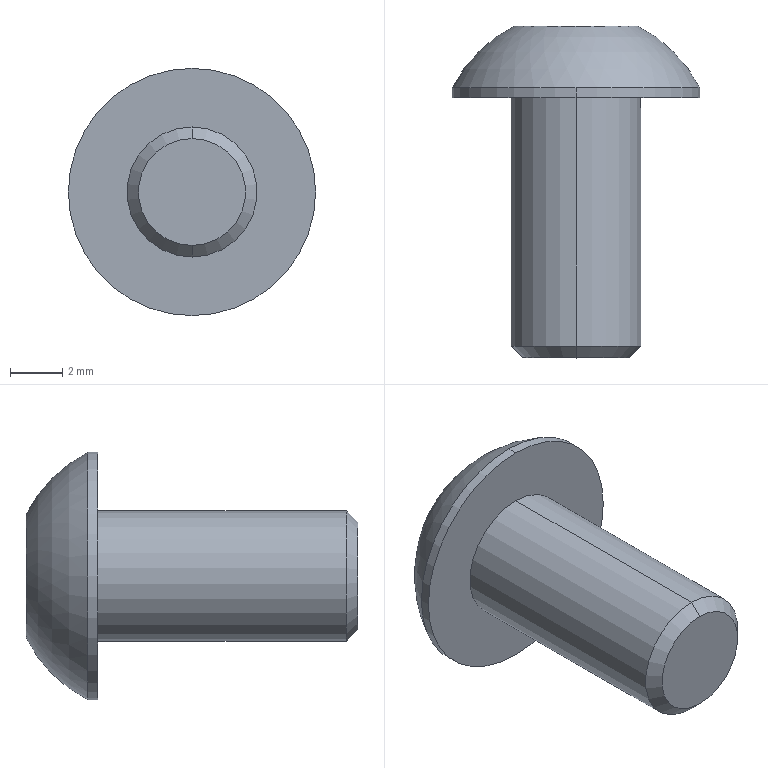Part | SolidWorks | features BaseBody 1 | 1 solid | 17 faces | box 9.5 x 12.75 x 9.5 mm | volume 321.053 mm3 | plane 10 | cylinder 4 | cone 2 | sphere 1 | commonest cylinder face diameters 5 x2 9.5 x2
STEP:
#1=CARTESIAN_POINT('',(0.,-10.,-2.055));
#2=VERTEX_POINT('',#1);
#3=CARTESIAN_POINT('',(0.,-10.,2.055));
#4=VERTEX_POINT('',#3);
#5=CARTESIAN_POINT('',(0.,-10.,0.));
#6=DIRECTION('',(0.,-1.,0.));
#7=DIRECTION('',(0.,0.,-1.));
#8=AXIS2_PLACEMENT_3D('',#5,#6,#7);
#9=CIRCLE('',#8,2.055);
#10=EDGE_CURVE('',#2,#4,#9,.T.);
#11=ORIENTED_EDGE('',*,*,#10,.F.);
#12=CARTESIAN_POINT('',(0.,-9.555,-2.5));
#13=VERTEX_POINT('',#12);
#14=CARTESIAN_POINT('',(0.,-10.,-2.055));
#15=DIRECTION('',(0.,0.7071,-0.7071));
#16=VECTOR('',#15,1000.);
#17=LINE('',#14,#16);
#18=EDGE_CURVE('',#2,#13,#17,.T.);
#19=ORIENTED_EDGE('',*,*,#18,.T.);
#20=CARTESIAN_POINT('',(0.,-9.555,2.5));
#21=VERTEX_POINT('',#20);
#22=CARTESIAN_POINT('',(0.,-9.555,0.));
#23=DIRECTION('',(0.,1.,0.));
#24=DIRECTION('',(0.,0.,-1.));
#25=AXIS2_PLACEMENT_3D('',#22,#23,#24);
#26=CIRCLE('',#25,2.5);
#27=EDGE_CURVE('',#21,#13,#26,.T.);
#28=ORIENTED_EDGE('',*,*,#27,.F.);
#29=CARTESIAN_POINT('',(0.,-10.,2.055));
#30=DIRECTION('',(0.,0.7071,0.7071));
#31=VECTOR('',#30,1000.);
#32=LINE('',#29,#31);
#33=EDGE_CURVE('',#4,#21,#32,.T.);
#34=ORIENTED_EDGE('',*,*,#33,.F.);
#35=EDGE_LOOP('',(#11,#19,#28,#34));
#36=FACE_OUTER_BOUND('',#35,.T.);
#37=CARTESIAN_POINT('',(0.,-10.,0.));
#38=DIRECTION('',(0.,1.,0.));
#39=DIRECTION('',(0.,0.,1.));
#40=AXIS2_PLACEMENT_3D('',#37,#38,#39);
#41=CONICAL_SURFACE('',#40,2.055,0.7854);
#42=ADVANCED_FACE('',(#36),#41,.T.);
#43=ORIENTED_EDGE('',*,*,#27,.T.);
#44=CARTESIAN_POINT('',(0.,0.,-2.5));
#45=VERTEX_POINT('',#44);
#46=CARTESIAN_POINT('',(0.,-10.,-2.5));
#47=DIRECTION('',(0.,1.,0.));
#48=VECTOR('',#47,1000.);
#49=LINE('',#46,#48);
#50=EDGE_CURVE('',#13,#45,#49,.T.);
#51=ORIENTED_EDGE('',*,*,#50,.T.);
#52=CARTESIAN_POINT('',(0.,0.,2.5));
#53=VERTEX_POINT('',#52);
#54=CARTESIAN_POINT('',(0.,0.,0.));
#55=DIRECTION('',(0.,-1.,0.));
#56=DIRECTION('',(0.,0.,1.));
#57=AXIS2_PLACEMENT_3D('',#54,#55,#56);
#58=CIRCLE('',#57,2.5);
#59=EDGE_CURVE('',#45,#53,#58,.T.);
#60=ORIENTED_EDGE('',*,*,#59,.T.);
#61=CARTESIAN_POINT('',(0.,-10.,2.5));
#62=DIRECTION('',(0.,1.,0.));
#63=VECTOR('',#62,1000.);
#64=LINE('',#61,#63);
#65=EDGE_CURVE('',#21,#53,#64,.T.);
#66=ORIENTED_EDGE('',*,*,#65,.F.);
#67=EDGE_LOOP('',(#43,#51,#60,#66));
#68=FACE_OUTER_BOUND('',#67,.T.);
#69=CARTESIAN_POINT('',(0.,-10.,0.));
#70=DIRECTION('',(0.,1.,0.));
#71=DIRECTION('',(0.,0.,1.));
#72=AXIS2_PLACEMENT_3D('',#69,#70,#71);
#73=CYLINDRICAL_SURFACE('',#72,2.5);
#74=ADVANCED_FACE('',(#68),#73,.T.);
#75=CARTESIAN_POINT('',(0.,0.38,-4.75));
#76=VERTEX_POINT('',#75);
#77=CARTESIAN_POINT('',(0.,0.38,4.75));
#78=VERTEX_POINT('',#77);
#79=CARTESIAN_POINT('',(0.,0.38,0.));
#80=DIRECTION('',(0.,-1.,0.));
#81=DIRECTION('',(0.,0.,-1.));
#82=AXIS2_PLACEMENT_3D('',#79,#80,#81);
#83=CIRCLE('',#82,4.75);
#84=EDGE_CURVE('',#76,#78,#83,.T.);
#85=ORIENTED_EDGE('',*,*,#84,.T.);
#86=CARTESIAN_POINT('',(0.,0.,4.75));
#87=VERTEX_POINT('',#86);
#88=CARTESIAN_POINT('',(0.,2.75,4.75));
#89=DIRECTION('',(0.,-1.,0.));
#90=VECTOR('',#89,1000.);
#91=LINE('',#88,#90);
#92=EDGE_CURVE('',#78,#87,#91,.T.);
#93=ORIENTED_EDGE('',*,*,#92,.T.);
#94=CARTESIAN_POINT('',(0.,0.,-4.75));
#95=VERTEX_POINT('',#94);
#96=CARTESIAN_POINT('',(0.,0.,0.));
#97=DIRECTION('',(0.,1.,0.));
#98=DIRECTION('',(0.,0.,1.));
#99=AXIS2_PLACEMENT_3D('',#96,#97,#98);
#100=CIRCLE('',#99,4.75);
#101=EDGE_CURVE('',#87,#95,#100,.T.);
#102=ORIENTED_EDGE('',*,*,#101,.T.);
#103=CARTESIAN_POINT('',(0.,2.75,-4.75));
#104=DIRECTION('',(0.,-1.,0.));
#105=VECTOR('',#104,1000.);
#106=LINE('',#103,#105);
#107=EDGE_CURVE('',#76,#95,#106,.T.);
#108=ORIENTED_EDGE('',*,*,#107,.F.);
#109=EDGE_LOOP('',(#85,#93,#102,#108));
#110=FACE_OUTER_BOUND('',#109,.T.);
#111=CARTESIAN_POINT('',(0.,2.75,0.));
#112=DIRECTION('',(0.,-1.,0.));
#113=DIRECTION('',(0.,0.,-1.));
#114=AXIS2_PLACEMENT_3D('',#111,#112,#113);
#115=CYLINDRICAL_SURFACE('',#114,4.75);
#116=ADVANCED_FACE('',(#110),#115,.T.);
#117=CARTESIAN_POINT('',(0.8862,2.75,1.535));
#118=VERTEX_POINT('',#117);
#119=CARTESIAN_POINT('',(1.772,2.75,0.));
#120=VERTEX_POINT('',#119);
#121=CARTESIAN_POINT('',(0.8862,2.75,1.535));
#122=DIRECTION('',(0.5,0.,-0.866));
#123=VECTOR('',#122,1000.);
#124=LINE('',#121,#123);
#125=EDGE_CURVE('',#118,#120,#124,.T.);
#126=ORIENTED_EDGE('',*,*,#125,.F.);
#127=CARTESIAN_POINT('',(-0.8862,2.75,1.535));
#128=VERTEX_POINT('',#127);
#129=CARTESIAN_POINT('',(-0.8862,2.75,1.535));
#130=DIRECTION('',(1.,0.,0.));
#131=VECTOR('',#130,1000.);
#132=LINE('',#129,#131);
#133=EDGE_CURVE('',#128,#118,#132,.T.);
#134=ORIENTED_EDGE('',*,*,#133,.F.);
#135=CARTESIAN_POINT('',(-1.772,2.75,0.));
#136=VERTEX_POINT('',#135);
#137=CARTESIAN_POINT('',(-1.772,2.75,0.));
#138=DIRECTION('',(0.5,0.,0.866));
#139=VECTOR('',#138,1000.);
#140=LINE('',#137,#139);
#141=EDGE_CURVE('',#136,#128,#140,.T.);
#142=ORIENTED_EDGE('',*,*,#141,.F.);
#143=CARTESIAN_POINT('',(-0.8862,2.75,-1.535));
#144=VERTEX_POINT('',#143);
#145=CARTESIAN_POINT('',(-0.8862,2.75,-1.535));
#146=DIRECTION('',(-0.5,0.,0.866));
#147=VECTOR('',#146,1000.);
#148=LINE('',#145,#147);
#149=EDGE_CURVE('',#144,#136,#148,.T.);
#150=ORIENTED_EDGE('',*,*,#149,.F.);
#151=CARTESIAN_POINT('',(0.8862,2.75,-1.535));
#152=VERTEX_POINT('',#151);
#153=CARTESIAN_POINT('',(0.8862,2.75,-1.535));
#154=DIRECTION('',(-1.,0.,0.));
#155=VECTOR('',#154,1000.);
#156=LINE('',#153,#155);
#157=EDGE_CURVE('',#152,#144,#156,.T.);
#158=ORIENTED_EDGE('',*,*,#157,.F.);
#159=CARTESIAN_POINT('',(1.772,2.75,0.));
#160=DIRECTION('',(-0.5,0.,-0.866));
#161=VECTOR('',#160,1000.);
#162=LINE('',#159,#161);
#163=EDGE_CURVE('',#120,#152,#162,.T.);
#164=ORIENTED_EDGE('',*,*,#163,.F.);
#165=EDGE_LOOP('',(#126,#134,#142,#150,#158,#164));
#166=FACE_BOUND('',#165,.T.);
#167=CARTESIAN_POINT('',(0.,2.75,-2.375));
#168=VERTEX_POINT('',#167);
#169=CARTESIAN_POINT('',(0.,2.75,2.375));
#170=VERTEX_POINT('',#169);
#171=CARTESIAN_POINT('',(0.,2.75,0.));
#172=DIRECTION('',(0.,-1.,0.));
#173=DIRECTION('',(0.,0.,-1.));
#174=AXIS2_PLACEMENT_3D('',#171,#172,#173);
#175=CIRCLE('',#174,2.375);
#176=EDGE_CURVE('',#168,#170,#175,.T.);
#177=ORIENTED_EDGE('',*,*,#176,.F.);
#178=CARTESIAN_POINT('',(0.,2.75,0.));
#179=DIRECTION('',(0.,-1.,0.));
#180=DIRECTION('',(0.,0.,-1.));
#181=AXIS2_PLACEMENT_3D('',#178,#179,#180);
#182=CIRCLE('',#181,2.375);
#183=EDGE_CURVE('',#170,#168,#182,.T.);
#184=ORIENTED_EDGE('',*,*,#183,.F.);
#185=EDGE_LOOP('',(#177,#184));
#186=FACE_OUTER_BOUND('',#185,.T.);
#187=CARTESIAN_POINT('',(0.,2.75,0.));
#188=DIRECTION('',(0.,1.,0.));
#189=DIRECTION('',(1.,0.,0.));
#190=AXIS2_PLACEMENT_3D('',#187,#188,#189);
#191=PLANE('',#190);
#192=ADVANCED_FACE('',(#166,#186),#191,.T.);
#193=ORIENTED_EDGE('',*,*,#125,.T.);
#194=CARTESIAN_POINT('',(1.772,1.19,0.));
#195=VERTEX_POINT('',#194);
#196=CARTESIAN_POINT('',(1.772,1.19,0.));
#197=DIRECTION('',(0.,1.,0.));
#198=VECTOR('',#197,1000.);
#199=LINE('',#196,#198);
#200=EDGE_CURVE('',#195,#120,#199,.T.);
#201=ORIENTED_EDGE('',*,*,#200,.F.);
#202=CARTESIAN_POINT('',(0.8862,1.19,1.535));
#203=VERTEX_POINT('',#202);
#204=CARTESIAN_POINT('',(0.8862,1.19,1.535));
#205=DIRECTION('',(0.5,0.,-0.866));
#206=VECTOR('',#205,1000.);
#207=LINE('',#204,#206);
#208=EDGE_CURVE('',#203,#195,#207,.T.);
#209=ORIENTED_EDGE('',*,*,#208,.F.);
#210=CARTESIAN_POINT('',(0.8862,1.19,1.535));
#211=DIRECTION('',(0.,1.,0.));
#212=VECTOR('',#211,1000.);
#213=LINE('',#210,#212);
#214=EDGE_CURVE('',#203,#118,#213,.T.);
#215=ORIENTED_EDGE('',*,*,#214,.T.);
#216=EDGE_LOOP('',(#193,#201,#209,#215));
#217=FACE_OUTER_BOUND('',#216,.T.);
#218=CARTESIAN_POINT('',(0.8862,1.19,1.535));
#219=DIRECTION('',(0.866,0.,0.5));
#220=DIRECTION('',(0.,-1.,0.));
#221=AXIS2_PLACEMENT_3D('',#218,#219,#220);
#222=PLANE('',#221);
#223=ADVANCED_FACE('',(#217),#222,.F.);
#224=ORIENTED_EDGE('',*,*,#133,.T.);
#225=ORIENTED_EDGE('',*,*,#214,.F.);
#226=CARTESIAN_POINT('',(-0.8862,1.19,1.535));
#227=VERTEX_POINT('',#226);
#228=CARTESIAN_POINT('',(-0.8862,1.19,1.535));
#229=DIRECTION('',(1.,0.,0.));
#230=VECTOR('',#229,1000.);
#231=LINE('',#228,#230);
#232=EDGE_CURVE('',#227,#203,#231,.T.);
#233=ORIENTED_EDGE('',*,*,#232,.F.);
#234=CARTESIAN_POINT('',(-0.8862,1.19,1.535));
#235=DIRECTION('',(0.,1.,0.));
#236=VECTOR('',#235,1000.);
#237=LINE('',#234,#236);
#238=EDGE_CURVE('',#227,#128,#237,.T.);
#239=ORIENTED_EDGE('',*,*,#238,.T.);
#240=EDGE_LOOP('',(#224,#225,#233,#239));
#241=FACE_OUTER_BOUND('',#240,.T.);
#242=CARTESIAN_POINT('',(-0.8862,1.19,1.535));
#243=DIRECTION('',(0.,0.,1.));
#244=DIRECTION('',(1.,0.,0.));
#245=AXIS2_PLACEMENT_3D('',#242,#243,#244);
#246=PLANE('',#245);
#247=ADVANCED_FACE('',(#241),#246,.F.);
#248=ORIENTED_EDGE('',*,*,#141,.T.);
#249=ORIENTED_EDGE('',*,*,#238,.F.);
#250=CARTESIAN_POINT('',(-1.772,1.19,0.));
#251=VERTEX_POINT('',#250);
#252=CARTESIAN_POINT('',(-1.772,1.19,0.));
#253=DIRECTION('',(0.5,0.,0.866));
#254=VECTOR('',#253,1000.);
#255=LINE('',#252,#254);
#256=EDGE_CURVE('',#251,#227,#255,.T.);
#257=ORIENTED_EDGE('',*,*,#256,.F.);
#258=CARTESIAN_POINT('',(-1.772,1.19,0.));
#259=DIRECTION('',(0.,1.,0.));
#260=VECTOR('',#259,1000.);
#261=LINE('',#258,#260);
#262=EDGE_CURVE('',#251,#136,#261,.T.);
#263=ORIENTED_EDGE('',*,*,#262,.T.);
#264=EDGE_LOOP('',(#248,#249,#257,#263));
#265=FACE_OUTER_BOUND('',#264,.T.);
#266=CARTESIAN_POINT('',(-1.772,1.19,0.));
#267=DIRECTION('',(-0.866,0.,0.5));
#268=DIRECTION('',(0.,1.,0.));
#269=AXIS2_PLACEMENT_3D('',#266,#267,#268);
#270=PLANE('',#269);
#271=ADVANCED_FACE('',(#265),#270,.F.);
#272=ORIENTED_EDGE('',*,*,#149,.T.);
#273=ORIENTED_EDGE('',*,*,#262,.F.);
#274=CARTESIAN_POINT('',(-0.8862,1.19,-1.535));
#275=VERTEX_POINT('',#274);
#276=CARTESIAN_POINT('',(-0.8862,1.19,-1.535));
#277=DIRECTION('',(-0.5,0.,0.866));
#278=VECTOR('',#277,1000.);
#279=LINE('',#276,#278);
#280=EDGE_CURVE('',#275,#251,#279,.T.);
#281=ORIENTED_EDGE('',*,*,#280,.F.);
#282=CARTESIAN_POINT('',(-0.8862,1.19,-1.535));
#283=DIRECTION('',(0.,1.,0.));
#284=VECTOR('',#283,1000.);
#285=LINE('',#282,#284);
#286=EDGE_CURVE('',#275,#144,#285,.T.);
#287=ORIENTED_EDGE('',*,*,#286,.T.);
#288=EDGE_LOOP('',(#272,#273,#281,#287));
#289=FACE_OUTER_BOUND('',#288,.T.);
#290=CARTESIAN_POINT('',(-0.8862,1.19,-1.535));
#291=DIRECTION('',(-0.866,0.,-0.5));
#292=DIRECTION('',(-0.5,0.,0.866));
#293=AXIS2_PLACEMENT_3D('',#290,#291,#292);
#294=PLANE('',#293);
#295=ADVANCED_FACE('',(#289),#294,.F.);
#296=ORIENTED_EDGE('',*,*,#157,.T.);
#297=ORIENTED_EDGE('',*,*,#286,.F.);
#298=CARTESIAN_POINT('',(0.8862,1.19,-1.535));
#299=VERTEX_POINT('',#298);
#300=CARTESIAN_POINT('',(0.8862,1.19,-1.535));
#301=DIRECTION('',(-1.,0.,0.));
#302=VECTOR('',#301,1000.);
#303=LINE('',#300,#302);
#304=EDGE_CURVE('',#299,#275,#303,.T.);
#305=ORIENTED_EDGE('',*,*,#304,.F.);
#306=CARTESIAN_POINT('',(0.8862,1.19,-1.535));
#307=DIRECTION('',(0.,1.,0.));
#308=VECTOR('',#307,1000.);
#309=LINE('',#306,#308);
#310=EDGE_CURVE('',#299,#152,#309,.T.);
#311=ORIENTED_EDGE('',*,*,#310,.T.);
#312=EDGE_LOOP('',(#296,#297,#305,#311));
#313=FACE_OUTER_BOUND('',#312,.T.);
#314=CARTESIAN_POINT('',(0.8862,1.19,-1.535));
#315=DIRECTION('',(0.,0.,-1.));
#316=DIRECTION('',(-1.,0.,0.));
#317=AXIS2_PLACEMENT_3D('',#314,#315,#316);
#318=PLANE('',#317);
#319=ADVANCED_FACE('',(#313),#318,.F.);
#320=ORIENTED_EDGE('',*,*,#163,.T.);
#321=ORIENTED_EDGE('',*,*,#310,.F.);
#322=CARTESIAN_POINT('',(1.772,1.19,0.));
#323=DIRECTION('',(-0.5,0.,-0.866));
#324=VECTOR('',#323,1000.);
#325=LINE('',#322,#324);
#326=EDGE_CURVE('',#195,#299,#325,.T.);
#327=ORIENTED_EDGE('',*,*,#326,.F.);
#328=ORIENTED_EDGE('',*,*,#200,.T.);
#329=EDGE_LOOP('',(#320,#321,#327,#328));
#330=FACE_OUTER_BOUND('',#329,.T.);
#331=CARTESIAN_POINT('',(1.772,1.19,0.));
#332=DIRECTION('',(0.866,0.,-0.5));
#333=DIRECTION('',(0.,-1.,0.));
#334=AXIS2_PLACEMENT_3D('',#331,#332,#333);
#335=PLANE('',#334);
#336=ADVANCED_FACE('',(#330),#335,.F.);
#337=ORIENTED_EDGE('',*,*,#208,.T.);
#338=ORIENTED_EDGE('',*,*,#326,.T.);
#339=ORIENTED_EDGE('',*,*,#304,.T.);
#340=ORIENTED_EDGE('',*,*,#280,.T.);
#341=ORIENTED_EDGE('',*,*,#256,.T.);
#342=ORIENTED_EDGE('',*,*,#232,.T.);
#343=EDGE_LOOP('',(#337,#338,#339,#340,#341,#342));
#344=FACE_OUTER_BOUND('',#343,.T.);
#345=CARTESIAN_POINT('',(0.,1.19,0.));
#346=DIRECTION('',(0.,1.,0.));
#347=DIRECTION('',(1.,0.,0.));
#348=AXIS2_PLACEMENT_3D('',#345,#346,#347);
#349=PLANE('',#348);
#350=ADVANCED_FACE('',(#344),#349,.T.);
#351=CARTESIAN_POINT('',(0.,-10.,0.));
#352=DIRECTION('',(0.,-1.,0.));
#353=DIRECTION('',(0.,0.,-1.));
#354=AXIS2_PLACEMENT_3D('',#351,#352,#353);
#355=CIRCLE('',#354,2.055);
#356=EDGE_CURVE('',#4,#2,#355,.T.);
#357=ORIENTED_EDGE('',*,*,#356,.T.);
#358=ORIENTED_EDGE('',*,*,#10,.T.);
#359=EDGE_LOOP('',(#357,#358));
#360=FACE_OUTER_BOUND('',#359,.T.);
#361=CARTESIAN_POINT('',(0.,-10.,0.));
#362=DIRECTION('',(0.,-1.,0.));
#363=DIRECTION('',(0.,0.,-1.));
#364=AXIS2_PLACEMENT_3D('',#361,#362,#363);
#365=PLANE('',#364);
#366=ADVANCED_FACE('',(#360),#365,.T.);
#367=CARTESIAN_POINT('',(0.,0.,0.));
#368=DIRECTION('',(0.,-1.,0.));
#369=DIRECTION('',(0.,0.,1.));
#370=AXIS2_PLACEMENT_3D('',#367,#368,#369);
#371=CIRCLE('',#370,2.5);
#372=EDGE_CURVE('',#53,#45,#371,.T.);
#373=ORIENTED_EDGE('',*,*,#372,.F.);
#374=ORIENTED_EDGE('',*,*,#59,.F.);
#375=EDGE_LOOP('',(#373,#374));
#376=FACE_BOUND('',#375,.T.);
#377=CARTESIAN_POINT('',(0.,0.,0.));
#378=DIRECTION('',(0.,1.,0.));
#379=DIRECTION('',(0.,0.,1.));
#380=AXIS2_PLACEMENT_3D('',#377,#378,#379);
#381=CIRCLE('',#380,4.75);
#382=EDGE_CURVE('',#95,#87,#381,.T.);
#383=ORIENTED_EDGE('',*,*,#382,.F.);
#384=ORIENTED_EDGE('',*,*,#101,.F.);
#385=EDGE_LOOP('',(#383,#384));
#386=FACE_OUTER_BOUND('',#385,.T.);
#387=CARTESIAN_POINT('',(0.,0.,0.));
#388=DIRECTION('',(0.,1.,0.));
#389=DIRECTION('',(1.,0.,0.));
#390=AXIS2_PLACEMENT_3D('',#387,#388,#389);
#391=PLANE('',#390);
#392=ADVANCED_FACE('',(#376,#386),#391,.F.);
#393=ORIENTED_EDGE('',*,*,#92,.F.);
#394=CARTESIAN_POINT('',(0.,0.38,0.));
#395=DIRECTION('',(0.,-1.,0.));
#396=DIRECTION('',(0.,0.,-1.));
#397=AXIS2_PLACEMENT_3D('',#394,#395,#396);
#398=CIRCLE('',#397,4.75);
#399=EDGE_CURVE('',#78,#76,#398,.T.);
#400=ORIENTED_EDGE('',*,*,#399,.T.);
#401=ORIENTED_EDGE('',*,*,#107,.T.);
#402=ORIENTED_EDGE('',*,*,#382,.T.);
#403=EDGE_LOOP('',(#393,#400,#401,#402));
#404=FACE_OUTER_BOUND('',#403,.T.);
#405=CARTESIAN_POINT('',(0.,2.75,0.));
#406=DIRECTION('',(0.,-1.,0.));
#407=DIRECTION('',(0.,0.,-1.));
#408=AXIS2_PLACEMENT_3D('',#405,#406,#407);
#409=CYLINDRICAL_SURFACE('',#408,4.75);
#410=ADVANCED_FACE('',(#404),#409,.T.);
#411=ORIENTED_EDGE('',*,*,#50,.F.);
#412=CARTESIAN_POINT('',(0.,-9.555,0.));
#413=DIRECTION('',(0.,1.,0.));
#414=DIRECTION('',(0.,0.,-1.));
#415=AXIS2_PLACEMENT_3D('',#412,#413,#414);
#416=CIRCLE('',#415,2.5);
#417=EDGE_CURVE('',#13,#21,#416,.T.);
#418=ORIENTED_EDGE('',*,*,#417,.T.);
#419=ORIENTED_EDGE('',*,*,#65,.T.);
#420=ORIENTED_EDGE('',*,*,#372,.T.);
#421=EDGE_LOOP('',(#411,#418,#419,#420));
#422=FACE_OUTER_BOUND('',#421,.T.);
#423=CARTESIAN_POINT('',(0.,-10.,0.));
#424=DIRECTION('',(0.,1.,0.));
#425=DIRECTION('',(0.,0.,1.));
#426=AXIS2_PLACEMENT_3D('',#423,#424,#425);
#427=CYLINDRICAL_SURFACE('',#426,2.5);
#428=ADVANCED_FACE('',(#422),#427,.T.);
#429=ORIENTED_EDGE('',*,*,#84,.F.);
#430=ORIENTED_EDGE('',*,*,#399,.F.);
#431=EDGE_LOOP('',(#429,#430));
#432=FACE_OUTER_BOUND('',#431,.T.);
#433=ORIENTED_EDGE('',*,*,#176,.T.);
#434=ORIENTED_EDGE('',*,*,#183,.T.);
#435=EDGE_LOOP('',(#433,#434));
#436=FACE_BOUND('',#435,.T.);
#437=CARTESIAN_POINT('',(0.,-2.005,0.));
#438=DIRECTION('',(0.,1.,0.));
#439=DIRECTION('',(1.,0.,0.));
#440=AXIS2_PLACEMENT_3D('',#437,#438,#439);
#441=SPHERICAL_SURFACE('',#440,5.315);
#442=ADVANCED_FACE('',(#432,#436),#441,.T.);
#443=ORIENTED_EDGE('',*,*,#18,.F.);
#444=ORIENTED_EDGE('',*,*,#356,.F.);
#445=ORIENTED_EDGE('',*,*,#33,.T.);
#446=ORIENTED_EDGE('',*,*,#417,.F.);
#447=EDGE_LOOP('',(#443,#444,#445,#446));
#448=FACE_OUTER_BOUND('',#447,.T.);
#449=CARTESIAN_POINT('',(0.,-10.,0.));
#450=DIRECTION('',(0.,1.,0.));
#451=DIRECTION('',(0.,0.,1.));
#452=AXIS2_PLACEMENT_3D('',#449,#450,#451);
#453=CONICAL_SURFACE('',#452,2.055,0.7854);
#454=ADVANCED_FACE('',(#448),#453,.T.);
#455=CLOSED_SHELL('',(#42,#74,#116,#192,#223,#247,#271,#295,#319,#336,#350,#366,#392,#410,#428,#442,#454));
#456=MANIFOLD_SOLID_BREP('',#455);
#457=CARTESIAN_POINT('',(0.,0.,0.));
#458=DIRECTION('',(0.,0.,1.));
#459=DIRECTION('',(1.,0.,0.));
#460=AXIS2_PLACEMENT_3D('',#457,#458,#459);
#461=(LENGTH_UNIT()NAMED_UNIT(*)SI_UNIT(.MILLI.,.METRE.));
#462=UNCERTAINTY_MEASURE_WITH_UNIT(LENGTH_MEASURE(0.00001),#461,'','');
#463=(NAMED_UNIT(*)PLANE_ANGLE_UNIT()SI_UNIT($,.RADIAN.));
#464=(NAMED_UNIT(*)SI_UNIT($,.STERADIAN.)SOLID_ANGLE_UNIT());
#465=(GEOMETRIC_REPRESENTATION_CONTEXT(3)GLOBAL_UNCERTAINTY_ASSIGNED_CONTEXT((#462))GLOBAL_UNIT_ASSIGNED_CONTEXT((#461,#463,#464))REPRESENTATION_CONTEXT('',''));
#466=ADVANCED_BREP_SHAPE_REPRESENTATION('',(#456,#460),#465);